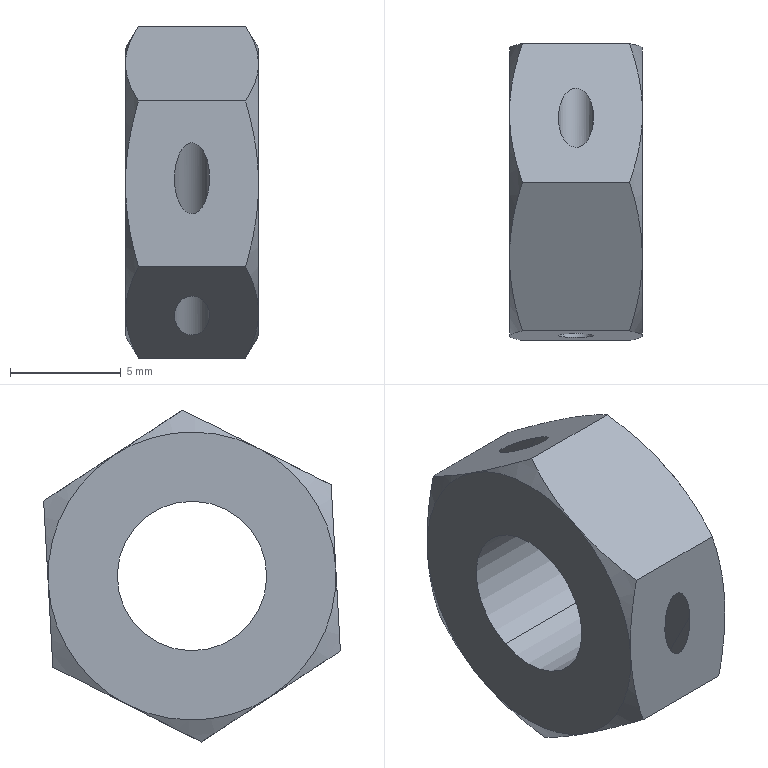Part | SolidWorks | features BaseBody 1 | 1 solid | 26 faces | box 6 x 13.398 x 14.988 mm | volume 630.737 mm3 | cone 12 | plane 8 | cylinder 6 | commonest cylinder face diameters 1.6 x4 6.75 x2
STEP:
#1=CARTESIAN_POINT('',(441.9,158.524,0.6198));
#2=VERTEX_POINT('',#1);
#3=CARTESIAN_POINT('',(440.3,158.524,0.6198));
#4=VERTEX_POINT('',#3);
#5=CARTESIAN_POINT('',(441.9,158.524,0.6198));
#6=CARTESIAN_POINT('',(441.9,158.346,-2.575));
#7=CARTESIAN_POINT('',(440.3,158.346,-2.575));
#8=CARTESIAN_POINT('',(440.3,158.524,0.6198));
#9=(BOUNDED_CURVE()B_SPLINE_CURVE(3,(#5,#6,#7,#8),.UNSPECIFIED.,.F.,.F.)B_SPLINE_CURVE_WITH_KNOTS((4,4),(4.712,7.854),.UNSPECIFIED.)CURVE()GEOMETRIC_REPRESENTATION_ITEM()RATIONAL_B_SPLINE_CURVE((1.,0.3333,0.3333,1.))REPRESENTATION_ITEM(''));
#10=EDGE_CURVE('',#2,#4,#9,.T.);
#11=ORIENTED_EDGE('',*,*,#10,.F.);
#12=CARTESIAN_POINT('',(441.9,161.658,-5.581));
#13=VERTEX_POINT('',#12);
#14=CARTESIAN_POINT('',(441.9,157.16,3.321));
#15=DIRECTION('',(0.,0.451,-0.8925));
#16=VECTOR('',#15,1000.);
#17=LINE('',#14,#16);
#18=EDGE_CURVE('',#2,#13,#17,.T.);
#19=ORIENTED_EDGE('',*,*,#18,.T.);
#20=CARTESIAN_POINT('',(440.3,161.658,-5.581));
#21=VERTEX_POINT('',#20);
#22=CARTESIAN_POINT('',(440.3,161.658,-5.581));
#23=CARTESIAN_POINT('',(440.3,158.98,-3.829));
#24=CARTESIAN_POINT('',(441.9,158.98,-3.829));
#25=CARTESIAN_POINT('',(441.9,161.658,-5.581));
#26=(BOUNDED_CURVE()B_SPLINE_CURVE(3,(#22,#23,#24,#25),.UNSPECIFIED.,.F.,.F.)B_SPLINE_CURVE_WITH_KNOTS((4,4),(1.571,4.712),.UNSPECIFIED.)CURVE()GEOMETRIC_REPRESENTATION_ITEM()RATIONAL_B_SPLINE_CURVE((1.,0.3333,0.3333,1.))REPRESENTATION_ITEM(''));
#27=EDGE_CURVE('',#21,#13,#26,.T.);
#28=ORIENTED_EDGE('',*,*,#27,.F.);
#29=CARTESIAN_POINT('',(440.3,157.16,3.321));
#30=DIRECTION('',(0.,0.451,-0.8925));
#31=VECTOR('',#30,1000.);
#32=LINE('',#29,#31);
#33=EDGE_CURVE('',#4,#21,#32,.T.);
#34=ORIENTED_EDGE('',*,*,#33,.F.);
#35=EDGE_LOOP('',(#11,#19,#28,#34));
#36=FACE_OUTER_BOUND('',#35,.T.);
#37=CARTESIAN_POINT('',(441.1,157.16,3.321));
#38=DIRECTION('',(0.,0.451,-0.8925));
#39=DIRECTION('',(-1.,0.,0.));
#40=AXIS2_PLACEMENT_3D('',#37,#38,#39);
#41=CYLINDRICAL_SURFACE('',#40,0.8);
#42=ADVANCED_FACE('',(#36),#41,.F.);
#43=CARTESIAN_POINT('',(441.9,168.342,5.581));
#44=VERTEX_POINT('',#43);
#45=CARTESIAN_POINT('',(440.3,168.342,5.581));
#46=VERTEX_POINT('',#45);
#47=CARTESIAN_POINT('',(441.9,168.342,5.581));
#48=CARTESIAN_POINT('',(441.9,165.664,7.333));
#49=CARTESIAN_POINT('',(440.3,165.664,7.333));
#50=CARTESIAN_POINT('',(440.3,168.342,5.581));
#51=(BOUNDED_CURVE()B_SPLINE_CURVE(3,(#47,#48,#49,#50),.UNSPECIFIED.,.F.,.T.)B_SPLINE_CURVE_WITH_KNOTS((4,4),(1.571,4.712),.UNSPECIFIED.)CURVE()GEOMETRIC_REPRESENTATION_ITEM()RATIONAL_B_SPLINE_CURVE((1.,0.3333,0.3333,1.))REPRESENTATION_ITEM(''));
#52=EDGE_CURVE('',#44,#46,#51,.T.);
#53=ORIENTED_EDGE('',*,*,#52,.F.);
#54=CARTESIAN_POINT('',(441.9,171.476,-0.6198));
#55=VERTEX_POINT('',#54);
#56=CARTESIAN_POINT('',(441.9,166.977,8.282));
#57=DIRECTION('',(0.,0.451,-0.8925));
#58=VECTOR('',#57,1000.);
#59=LINE('',#56,#58);
#60=EDGE_CURVE('',#44,#55,#59,.T.);
#61=ORIENTED_EDGE('',*,*,#60,.T.);
#62=CARTESIAN_POINT('',(440.3,171.476,-0.6198));
#63=VERTEX_POINT('',#62);
#64=CARTESIAN_POINT('',(440.3,171.476,-0.6198));
#65=CARTESIAN_POINT('',(440.3,171.297,-3.815));
#66=CARTESIAN_POINT('',(441.9,171.297,-3.815));
#67=CARTESIAN_POINT('',(441.9,171.476,-0.6198));
#68=(BOUNDED_CURVE()B_SPLINE_CURVE(3,(#64,#65,#66,#67),.UNSPECIFIED.,.F.,.T.)B_SPLINE_CURVE_WITH_KNOTS((4,4),(4.712,7.854),.UNSPECIFIED.)CURVE()GEOMETRIC_REPRESENTATION_ITEM()RATIONAL_B_SPLINE_CURVE((1.,0.3333,0.3333,1.))REPRESENTATION_ITEM(''));
#69=EDGE_CURVE('',#63,#55,#68,.T.);
#70=ORIENTED_EDGE('',*,*,#69,.F.);
#71=CARTESIAN_POINT('',(440.3,166.977,8.282));
#72=DIRECTION('',(0.,0.451,-0.8925));
#73=VECTOR('',#72,1000.);
#74=LINE('',#71,#73);
#75=EDGE_CURVE('',#46,#63,#74,.T.);
#76=ORIENTED_EDGE('',*,*,#75,.F.);
#77=EDGE_LOOP('',(#53,#61,#70,#76));
#78=FACE_OUTER_BOUND('',#77,.T.);
#79=CARTESIAN_POINT('',(441.1,166.977,8.282));
#80=DIRECTION('',(0.,0.451,-0.8925));
#81=DIRECTION('',(-1.,0.,0.));
#82=AXIS2_PLACEMENT_3D('',#79,#80,#81);
#83=CYLINDRICAL_SURFACE('',#82,0.8);
#84=ADVANCED_FACE('',(#78),#83,.F.);
#85=CARTESIAN_POINT('',(438.1,163.478,3.012));
#86=VERTEX_POINT('',#85);
#87=CARTESIAN_POINT('',(438.1,166.522,-3.012));
#88=VERTEX_POINT('',#87);
#89=CARTESIAN_POINT('',(438.1,165.,0.));
#90=DIRECTION('',(1.,0.,0.));
#91=DIRECTION('',(0.,0.451,-0.8925));
#92=AXIS2_PLACEMENT_3D('',#89,#90,#91);
#93=CIRCLE('',#92,3.375);
#94=EDGE_CURVE('',#86,#88,#93,.T.);
#95=ORIENTED_EDGE('',*,*,#94,.F.);
#96=CARTESIAN_POINT('',(444.1,163.478,3.012));
#97=VERTEX_POINT('',#96);
#98=CARTESIAN_POINT('',(438.1,163.478,3.012));
#99=DIRECTION('',(1.,0.,0.));
#100=VECTOR('',#99,1000.);
#101=LINE('',#98,#100);
#102=EDGE_CURVE('',#86,#97,#101,.T.);
#103=ORIENTED_EDGE('',*,*,#102,.T.);
#104=CARTESIAN_POINT('',(444.1,166.522,-3.012));
#105=VERTEX_POINT('',#104);
#106=CARTESIAN_POINT('',(444.1,165.,0.));
#107=DIRECTION('',(1.,0.,0.));
#108=DIRECTION('',(0.,0.451,-0.8925));
#109=AXIS2_PLACEMENT_3D('',#106,#107,#108);
#110=CIRCLE('',#109,3.375);
#111=EDGE_CURVE('',#97,#105,#110,.T.);
#112=ORIENTED_EDGE('',*,*,#111,.T.);
#113=CARTESIAN_POINT('',(438.1,166.522,-3.012));
#114=DIRECTION('',(1.,0.,0.));
#115=VECTOR('',#114,1000.);
#116=LINE('',#113,#115);
#117=EDGE_CURVE('',#88,#105,#116,.T.);
#118=ORIENTED_EDGE('',*,*,#117,.F.);
#119=EDGE_LOOP('',(#95,#103,#112,#118));
#120=FACE_OUTER_BOUND('',#119,.T.);
#121=CARTESIAN_POINT('',(438.1,165.,0.));
#122=DIRECTION('',(1.,0.,0.));
#123=DIRECTION('',(0.,0.451,-0.8925));
#124=AXIS2_PLACEMENT_3D('',#121,#122,#123);
#125=CYLINDRICAL_SURFACE('',#124,3.375);
#126=ADVANCED_FACE('',(#120),#125,.F.);
#127=ORIENTED_EDGE('',*,*,#69,.T.);
#128=CARTESIAN_POINT('',(441.9,171.476,-0.6198));
#129=CARTESIAN_POINT('',(441.9,171.654,2.575));
#130=CARTESIAN_POINT('',(440.3,171.654,2.575));
#131=CARTESIAN_POINT('',(440.3,171.476,-0.6198));
#132=(BOUNDED_CURVE()B_SPLINE_CURVE(3,(#128,#129,#130,#131),.UNSPECIFIED.,.F.,.F.)B_SPLINE_CURVE_WITH_KNOTS((4,4),(1.571,4.712),.UNSPECIFIED.)CURVE()GEOMETRIC_REPRESENTATION_ITEM()RATIONAL_B_SPLINE_CURVE((1.,0.3333,0.3333,1.))REPRESENTATION_ITEM(''));
#133=EDGE_CURVE('',#55,#63,#132,.T.);
#134=ORIENTED_EDGE('',*,*,#133,.T.);
#135=EDGE_LOOP('',(#127,#134));
#136=FACE_BOUND('',#135,.T.);
#137=CARTESIAN_POINT('',(438.681,171.699,3.385));
#138=VERTEX_POINT('',#137);
#139=CARTESIAN_POINT('',(438.1,171.49,-0.3619));
#140=VERTEX_POINT('',#139);
#141=CARTESIAN_POINT('',(438.681,171.699,3.385));
#142=CARTESIAN_POINT('',(438.503,171.665,2.772));
#143=CARTESIAN_POINT('',(438.357,171.63,2.155));
#144=CARTESIAN_POINT('',(438.155,171.561,0.9069));
#145=CARTESIAN_POINT('',(438.1,171.526,0.2765));
#146=CARTESIAN_POINT('',(438.1,171.49,-0.3619));
#147=B_SPLINE_CURVE_WITH_KNOTS('',3,(#141,#142,#143,#144,#145,#146),.UNSPECIFIED.,.F.,.F.,(4,2,4),(0.000000238,0.001899,0.003797),.UNSPECIFIED.);
#148=EDGE_CURVE('',#138,#140,#147,.T.);
#149=ORIENTED_EDGE('',*,*,#148,.F.);
#150=CARTESIAN_POINT('',(443.519,171.699,3.385));
#151=VERTEX_POINT('',#150);
#152=CARTESIAN_POINT('',(444.1,171.699,3.385));
#153=DIRECTION('',(-1.,0.,0.));
#154=VECTOR('',#153,1000.);
#155=LINE('',#152,#154);
#156=EDGE_CURVE('',#151,#138,#155,.T.);
#157=ORIENTED_EDGE('',*,*,#156,.F.);
#158=CARTESIAN_POINT('',(444.1,171.49,-0.3619));
#159=VERTEX_POINT('',#158);
#160=CARTESIAN_POINT('',(444.1,171.49,-0.3619));
#161=CARTESIAN_POINT('',(444.1,171.508,-0.04387));
#162=CARTESIAN_POINT('',(444.086,171.525,0.2755));
#163=CARTESIAN_POINT('',(444.033,171.561,0.9074));
#164=CARTESIAN_POINT('',(443.994,171.578,1.221));
#165=CARTESIAN_POINT('',(443.842,171.63,2.157));
#166=CARTESIAN_POINT('',(443.696,171.665,2.774));
#167=CARTESIAN_POINT('',(443.519,171.699,3.385));
#168=B_SPLINE_CURVE_WITH_KNOTS('',3,(#160,#161,#162,#163,#164,#165,#166,#167),.UNSPECIFIED.,.F.,.F.,(4,2,2,4),(0.003797,0.004743,0.005689,0.00758),.UNSPECIFIED.);
#169=EDGE_CURVE('',#159,#151,#168,.T.);
#170=ORIENTED_EDGE('',*,*,#169,.F.);
#171=CARTESIAN_POINT('',(443.519,171.281,-4.109));
#172=VERTEX_POINT('',#171);
#173=CARTESIAN_POINT('',(443.519,171.281,-4.109));
#174=CARTESIAN_POINT('',(443.697,171.315,-3.496));
#175=CARTESIAN_POINT('',(443.843,171.35,-2.878));
#176=CARTESIAN_POINT('',(444.045,171.419,-1.631));
#177=CARTESIAN_POINT('',(444.1,171.454,-1.));
#178=CARTESIAN_POINT('',(444.1,171.49,-0.3619));
#179=B_SPLINE_CURVE_WITH_KNOTS('',3,(#173,#174,#175,#176,#177,#178),.UNSPECIFIED.,.F.,.F.,(4,2,4),(0.000000238,0.001899,0.003797),.UNSPECIFIED.);
#180=EDGE_CURVE('',#172,#159,#179,.T.);
#181=ORIENTED_EDGE('',*,*,#180,.F.);
#182=CARTESIAN_POINT('',(438.681,171.281,-4.109));
#183=VERTEX_POINT('',#182);
#184=CARTESIAN_POINT('',(444.1,171.281,-4.109));
#185=DIRECTION('',(-1.,0.,0.));
#186=VECTOR('',#185,1000.);
#187=LINE('',#184,#186);
#188=EDGE_CURVE('',#172,#183,#187,.T.);
#189=ORIENTED_EDGE('',*,*,#188,.T.);
#190=CARTESIAN_POINT('',(438.1,171.49,-0.3619));
#191=CARTESIAN_POINT('',(438.1,171.472,-0.6799));
#192=CARTESIAN_POINT('',(438.114,171.454,-0.9993));
#193=CARTESIAN_POINT('',(438.167,171.419,-1.631));
#194=CARTESIAN_POINT('',(438.206,171.402,-1.945));
#195=CARTESIAN_POINT('',(438.358,171.349,-2.881));
#196=CARTESIAN_POINT('',(438.504,171.315,-3.497));
#197=CARTESIAN_POINT('',(438.681,171.281,-4.109));
#198=B_SPLINE_CURVE_WITH_KNOTS('',3,(#190,#191,#192,#193,#194,#195,#196,#197),.UNSPECIFIED.,.F.,.F.,(4,2,2,4),(0.003797,0.004743,0.005689,0.00758),.UNSPECIFIED.);
#199=EDGE_CURVE('',#140,#183,#198,.T.);
#200=ORIENTED_EDGE('',*,*,#199,.F.);
#201=EDGE_LOOP('',(#149,#157,#170,#181,#189,#200));
#202=FACE_OUTER_BOUND('',#201,.T.);
#203=CARTESIAN_POINT('',(444.1,171.281,-4.109));
#204=DIRECTION('',(0.,-0.9984,0.05567));
#205=DIRECTION('',(0.,-0.05567,-0.9984));
#206=AXIS2_PLACEMENT_3D('',#203,#204,#205);
#207=PLANE('',#206);
#208=ADVANCED_FACE('',(#136,#202),#207,.F.);
#209=CARTESIAN_POINT('',(440.3,168.342,5.581));
#210=CARTESIAN_POINT('',(440.3,171.02,3.829));
#211=CARTESIAN_POINT('',(441.9,171.02,3.829));
#212=CARTESIAN_POINT('',(441.9,168.342,5.581));
#213=(BOUNDED_CURVE()B_SPLINE_CURVE(3,(#209,#210,#211,#212),.UNSPECIFIED.,.F.,.F.)B_SPLINE_CURVE_WITH_KNOTS((4,4),(4.712,7.854),.UNSPECIFIED.)CURVE()GEOMETRIC_REPRESENTATION_ITEM()RATIONAL_B_SPLINE_CURVE((1.,0.3333,0.3333,1.))REPRESENTATION_ITEM(''));
#214=EDGE_CURVE('',#46,#44,#213,.T.);
#215=ORIENTED_EDGE('',*,*,#214,.T.);
#216=ORIENTED_EDGE('',*,*,#52,.T.);
#217=EDGE_LOOP('',(#215,#216));
#218=FACE_BOUND('',#217,.T.);
#219=CARTESIAN_POINT('',(438.681,165.418,7.494));
#220=VERTEX_POINT('',#219);
#221=CARTESIAN_POINT('',(438.1,168.558,5.44));
#222=VERTEX_POINT('',#221);
#223=CARTESIAN_POINT('',(438.681,165.418,7.494));
#224=CARTESIAN_POINT('',(438.503,165.932,7.158));
#225=CARTESIAN_POINT('',(438.357,166.449,6.819));
#226=CARTESIAN_POINT('',(438.155,167.495,6.135));
#227=CARTESIAN_POINT('',(438.1,168.023,5.79));
#228=CARTESIAN_POINT('',(438.1,168.558,5.44));
#229=B_SPLINE_CURVE_WITH_KNOTS('',3,(#223,#224,#225,#226,#227,#228),.UNSPECIFIED.,.F.,.F.,(4,2,4),(0.000000238,0.001899,0.003797),.UNSPECIFIED.);
#230=EDGE_CURVE('',#220,#222,#229,.T.);
#231=ORIENTED_EDGE('',*,*,#230,.F.);
#232=CARTESIAN_POINT('',(443.519,165.418,7.494));
#233=VERTEX_POINT('',#232);
#234=CARTESIAN_POINT('',(444.1,165.418,7.494));
#235=DIRECTION('',(-1.,0.,0.));
#236=VECTOR('',#235,1000.);
#237=LINE('',#234,#236);
#238=EDGE_CURVE('',#233,#220,#237,.T.);
#239=ORIENTED_EDGE('',*,*,#238,.F.);
#240=CARTESIAN_POINT('',(444.1,168.558,5.44));
#241=VERTEX_POINT('',#240);
#242=CARTESIAN_POINT('',(444.1,168.558,5.44));
#243=CARTESIAN_POINT('',(444.1,168.292,5.614));
#244=CARTESIAN_POINT('',(444.086,168.024,5.789));
#245=CARTESIAN_POINT('',(444.033,167.494,6.135));
#246=CARTESIAN_POINT('',(443.994,167.231,6.308));
#247=CARTESIAN_POINT('',(443.842,166.447,6.821));
#248=CARTESIAN_POINT('',(443.696,165.93,7.159));
#249=CARTESIAN_POINT('',(443.519,165.418,7.494));
#250=B_SPLINE_CURVE_WITH_KNOTS('',3,(#242,#243,#244,#245,#246,#247,#248,#249),.UNSPECIFIED.,.F.,.F.,(4,2,2,4),(0.003797,0.004743,0.005689,0.00758),.UNSPECIFIED.);
#251=EDGE_CURVE('',#241,#233,#250,.T.);
#252=ORIENTED_EDGE('',*,*,#251,.F.);
#253=CARTESIAN_POINT('',(443.519,171.699,3.385));
#254=CARTESIAN_POINT('',(443.697,171.185,3.721));
#255=CARTESIAN_POINT('',(443.843,170.668,4.06));
#256=CARTESIAN_POINT('',(444.045,169.622,4.744));
#257=CARTESIAN_POINT('',(444.1,169.093,5.089));
#258=CARTESIAN_POINT('',(444.1,168.558,5.44));
#259=B_SPLINE_CURVE_WITH_KNOTS('',3,(#253,#254,#255,#256,#257,#258),.UNSPECIFIED.,.F.,.F.,(4,2,4),(0.000000238,0.001899,0.003797),.UNSPECIFIED.);
#260=EDGE_CURVE('',#151,#241,#259,.T.);
#261=ORIENTED_EDGE('',*,*,#260,.F.);
#262=ORIENTED_EDGE('',*,*,#156,.T.);
#263=CARTESIAN_POINT('',(438.1,168.558,5.44));
#264=CARTESIAN_POINT('',(438.1,168.825,5.265));
#265=CARTESIAN_POINT('',(438.114,169.093,5.09));
#266=CARTESIAN_POINT('',(438.167,169.622,4.744));
#267=CARTESIAN_POINT('',(438.206,169.885,4.572));
#268=CARTESIAN_POINT('',(438.358,170.67,4.058));
#269=CARTESIAN_POINT('',(438.504,171.186,3.72));
#270=CARTESIAN_POINT('',(438.681,171.699,3.385));
#271=B_SPLINE_CURVE_WITH_KNOTS('',3,(#263,#264,#265,#266,#267,#268,#269,#270),.UNSPECIFIED.,.F.,.F.,(4,2,2,4),(0.003797,0.004743,0.005689,0.00758),.UNSPECIFIED.);
#272=EDGE_CURVE('',#222,#138,#271,.T.);
#273=ORIENTED_EDGE('',*,*,#272,.F.);
#274=EDGE_LOOP('',(#231,#239,#252,#261,#262,#273));
#275=FACE_OUTER_BOUND('',#274,.T.);
#276=CARTESIAN_POINT('',(444.1,171.699,3.385));
#277=DIRECTION('',(0.,-0.5474,-0.8368));
#278=DIRECTION('',(0.,0.8368,-0.5474));
#279=AXIS2_PLACEMENT_3D('',#276,#277,#278);
#280=PLANE('',#279);
#281=ADVANCED_FACE('',(#218,#275),#280,.F.);
#282=CARTESIAN_POINT('',(438.681,158.719,4.109));
#283=VERTEX_POINT('',#282);
#284=CARTESIAN_POINT('',(438.1,162.068,5.801));
#285=VERTEX_POINT('',#284);
#286=CARTESIAN_POINT('',(438.681,158.719,4.109));
#287=CARTESIAN_POINT('',(438.504,159.265,4.385));
#288=CARTESIAN_POINT('',(438.357,159.822,4.666));
#289=CARTESIAN_POINT('',(438.155,160.939,5.231));
#290=CARTESIAN_POINT('',(438.1,161.501,5.515));
#291=CARTESIAN_POINT('',(438.1,162.068,5.801));
#292=B_SPLINE_CURVE_WITH_KNOTS('',3,(#286,#287,#288,#289,#290,#291),.UNSPECIFIED.,.F.,.F.,(4,2,4),(0.007046,0.008945,0.01085),.UNSPECIFIED.);
#293=EDGE_CURVE('',#283,#285,#292,.T.);
#294=ORIENTED_EDGE('',*,*,#293,.F.);
#295=CARTESIAN_POINT('',(443.519,158.719,4.109));
#296=VERTEX_POINT('',#295);
#297=CARTESIAN_POINT('',(444.1,158.719,4.109));
#298=DIRECTION('',(-1.,0.,0.));
#299=VECTOR('',#298,1000.);
#300=LINE('',#297,#299);
#301=EDGE_CURVE('',#296,#283,#300,.T.);
#302=ORIENTED_EDGE('',*,*,#301,.F.);
#303=CARTESIAN_POINT('',(444.1,162.068,5.801));
#304=VERTEX_POINT('',#303);
#305=CARTESIAN_POINT('',(444.1,162.068,5.801));
#306=CARTESIAN_POINT('',(444.1,161.501,5.515));
#307=CARTESIAN_POINT('',(444.045,160.939,5.231));
#308=CARTESIAN_POINT('',(443.843,159.822,4.666));
#309=CARTESIAN_POINT('',(443.696,159.265,4.385));
#310=CARTESIAN_POINT('',(443.519,158.719,4.109));
#311=B_SPLINE_CURVE_WITH_KNOTS('',3,(#305,#306,#307,#308,#309,#310),.UNSPECIFIED.,.F.,.F.,(4,2,4),(0.02413,0.02603,0.02793),.UNSPECIFIED.);
#312=EDGE_CURVE('',#304,#296,#311,.T.);
#313=ORIENTED_EDGE('',*,*,#312,.F.);
#314=CARTESIAN_POINT('',(443.519,165.418,7.494));
#315=CARTESIAN_POINT('',(443.695,164.876,7.22));
#316=CARTESIAN_POINT('',(443.84,164.327,6.943));
#317=CARTESIAN_POINT('',(443.993,163.489,6.519));
#318=CARTESIAN_POINT('',(444.033,163.208,6.377));
#319=CARTESIAN_POINT('',(444.086,162.638,6.089));
#320=CARTESIAN_POINT('',(444.1,162.352,5.945));
#321=CARTESIAN_POINT('',(444.1,162.068,5.801));
#322=B_SPLINE_CURVE_WITH_KNOTS('',3,(#314,#315,#316,#317,#318,#319,#320,#321),.UNSPECIFIED.,.F.,.F.,(4,2,2,4),(0.02033,0.02223,0.02318,0.02413),.UNSPECIFIED.);
#323=EDGE_CURVE('',#233,#304,#322,.T.);
#324=ORIENTED_EDGE('',*,*,#323,.F.);
#325=ORIENTED_EDGE('',*,*,#238,.T.);
#326=CARTESIAN_POINT('',(438.1,162.068,5.801));
#327=CARTESIAN_POINT('',(438.1,162.352,5.945));
#328=CARTESIAN_POINT('',(438.114,162.638,6.089));
#329=CARTESIAN_POINT('',(438.167,163.208,6.377));
#330=CARTESIAN_POINT('',(438.207,163.489,6.519));
#331=CARTESIAN_POINT('',(438.36,164.327,6.943));
#332=CARTESIAN_POINT('',(438.505,164.876,7.22));
#333=CARTESIAN_POINT('',(438.681,165.418,7.494));
#334=B_SPLINE_CURVE_WITH_KNOTS('',3,(#326,#327,#328,#329,#330,#331,#332,#333),.UNSPECIFIED.,.F.,.F.,(4,2,2,4),(0.01085,0.0118,0.01275,0.01465),.UNSPECIFIED.);
#335=EDGE_CURVE('',#285,#220,#334,.T.);
#336=ORIENTED_EDGE('',*,*,#335,.F.);
#337=EDGE_LOOP('',(#294,#302,#313,#324,#325,#336));
#338=FACE_OUTER_BOUND('',#337,.T.);
#339=CARTESIAN_POINT('',(444.1,165.418,7.494));
#340=DIRECTION('',(0.,0.451,-0.8925));
#341=DIRECTION('',(0.,0.8925,0.451));
#342=AXIS2_PLACEMENT_3D('',#339,#340,#341);
#343=PLANE('',#342);
#344=ADVANCED_FACE('',(#338),#343,.F.);
#345=CARTESIAN_POINT('',(440.3,158.524,0.6198));
#346=CARTESIAN_POINT('',(440.3,158.703,3.815));
#347=CARTESIAN_POINT('',(441.9,158.703,3.815));
#348=CARTESIAN_POINT('',(441.9,158.524,0.6198));
#349=(BOUNDED_CURVE()B_SPLINE_CURVE(3,(#345,#346,#347,#348),.UNSPECIFIED.,.F.,.F.)B_SPLINE_CURVE_WITH_KNOTS((4,4),(1.571,4.712),.UNSPECIFIED.)CURVE()GEOMETRIC_REPRESENTATION_ITEM()RATIONAL_B_SPLINE_CURVE((1.,0.3333,0.3333,1.))REPRESENTATION_ITEM(''));
#350=EDGE_CURVE('',#4,#2,#349,.T.);
#351=ORIENTED_EDGE('',*,*,#350,.T.);
#352=ORIENTED_EDGE('',*,*,#10,.T.);
#353=EDGE_LOOP('',(#351,#352));
#354=FACE_BOUND('',#353,.T.);
#355=CARTESIAN_POINT('',(438.681,158.301,-3.385));
#356=VERTEX_POINT('',#355);
#357=CARTESIAN_POINT('',(438.1,158.51,0.3619));
#358=VERTEX_POINT('',#357);
#359=CARTESIAN_POINT('',(438.681,158.301,-3.385));
#360=CARTESIAN_POINT('',(438.503,158.335,-2.772));
#361=CARTESIAN_POINT('',(438.357,158.37,-2.155));
#362=CARTESIAN_POINT('',(438.155,158.439,-0.9069));
#363=CARTESIAN_POINT('',(438.1,158.474,-0.2765));
#364=CARTESIAN_POINT('',(438.1,158.51,0.3619));
#365=B_SPLINE_CURVE_WITH_KNOTS('',3,(#359,#360,#361,#362,#363,#364),.UNSPECIFIED.,.F.,.F.,(4,2,4),(0.000000238,0.001899,0.003797),.UNSPECIFIED.);
#366=EDGE_CURVE('',#356,#358,#365,.T.);
#367=ORIENTED_EDGE('',*,*,#366,.F.);
#368=CARTESIAN_POINT('',(443.519,158.301,-3.385));
#369=VERTEX_POINT('',#368);
#370=CARTESIAN_POINT('',(444.1,158.301,-3.385));
#371=DIRECTION('',(-1.,0.,0.));
#372=VECTOR('',#371,1000.);
#373=LINE('',#370,#372);
#374=EDGE_CURVE('',#369,#356,#373,.T.);
#375=ORIENTED_EDGE('',*,*,#374,.F.);
#376=CARTESIAN_POINT('',(444.1,158.51,0.3619));
#377=VERTEX_POINT('',#376);
#378=CARTESIAN_POINT('',(444.1,158.51,0.3619));
#379=CARTESIAN_POINT('',(444.1,158.492,0.04387));
#380=CARTESIAN_POINT('',(444.086,158.475,-0.2755));
#381=CARTESIAN_POINT('',(444.033,158.439,-0.9074));
#382=CARTESIAN_POINT('',(443.994,158.422,-1.221));
#383=CARTESIAN_POINT('',(443.842,158.37,-2.157));
#384=CARTESIAN_POINT('',(443.696,158.335,-2.774));
#385=CARTESIAN_POINT('',(443.519,158.301,-3.385));
#386=B_SPLINE_CURVE_WITH_KNOTS('',3,(#378,#379,#380,#381,#382,#383,#384,#385),.UNSPECIFIED.,.F.,.F.,(4,2,2,4),(0.003797,0.004743,0.005689,0.00758),.UNSPECIFIED.);
#387=EDGE_CURVE('',#377,#369,#386,.T.);
#388=ORIENTED_EDGE('',*,*,#387,.F.);
#389=CARTESIAN_POINT('',(443.519,158.719,4.109));
#390=CARTESIAN_POINT('',(443.697,158.685,3.496));
#391=CARTESIAN_POINT('',(443.843,158.65,2.878));
#392=CARTESIAN_POINT('',(444.045,158.581,1.631));
#393=CARTESIAN_POINT('',(444.1,158.546,1.));
#394=CARTESIAN_POINT('',(444.1,158.51,0.3619));
#395=B_SPLINE_CURVE_WITH_KNOTS('',3,(#389,#390,#391,#392,#393,#394),.UNSPECIFIED.,.F.,.F.,(4,2,4),(0.000000238,0.001899,0.003797),.UNSPECIFIED.);
#396=EDGE_CURVE('',#296,#377,#395,.T.);
#397=ORIENTED_EDGE('',*,*,#396,.F.);
#398=ORIENTED_EDGE('',*,*,#301,.T.);
#399=CARTESIAN_POINT('',(438.1,158.51,0.3619));
#400=CARTESIAN_POINT('',(438.1,158.528,0.6799));
#401=CARTESIAN_POINT('',(438.114,158.546,0.9993));
#402=CARTESIAN_POINT('',(438.167,158.581,1.631));
#403=CARTESIAN_POINT('',(438.206,158.598,1.945));
#404=CARTESIAN_POINT('',(438.358,158.651,2.881));
#405=CARTESIAN_POINT('',(438.504,158.685,3.497));
#406=CARTESIAN_POINT('',(438.681,158.719,4.109));
#407=B_SPLINE_CURVE_WITH_KNOTS('',3,(#399,#400,#401,#402,#403,#404,#405,#406),.UNSPECIFIED.,.F.,.F.,(4,2,2,4),(0.003797,0.004743,0.005689,0.00758),.UNSPECIFIED.);
#408=EDGE_CURVE('',#358,#283,#407,.T.);
#409=ORIENTED_EDGE('',*,*,#408,.F.);
#410=EDGE_LOOP('',(#367,#375,#388,#397,#398,#409));
#411=FACE_OUTER_BOUND('',#410,.T.);
#412=CARTESIAN_POINT('',(444.1,158.719,4.109));
#413=DIRECTION('',(0.,0.9984,-0.05567));
#414=DIRECTION('',(0.,0.05567,0.9984));
#415=AXIS2_PLACEMENT_3D('',#412,#413,#414);
#416=PLANE('',#415);
#417=ADVANCED_FACE('',(#354,#411),#416,.F.);
#418=ORIENTED_EDGE('',*,*,#27,.T.);
#419=CARTESIAN_POINT('',(441.9,161.658,-5.581));
#420=CARTESIAN_POINT('',(441.9,164.336,-7.333));
#421=CARTESIAN_POINT('',(440.3,164.336,-7.333));
#422=CARTESIAN_POINT('',(440.3,161.658,-5.581));
#423=(BOUNDED_CURVE()B_SPLINE_CURVE(3,(#419,#420,#421,#422),.UNSPECIFIED.,.F.,.T.)B_SPLINE_CURVE_WITH_KNOTS((4,4),(4.712,7.854),.UNSPECIFIED.)CURVE()GEOMETRIC_REPRESENTATION_ITEM()RATIONAL_B_SPLINE_CURVE((1.,0.3333,0.3333,1.))REPRESENTATION_ITEM(''));
#424=EDGE_CURVE('',#13,#21,#423,.T.);
#425=ORIENTED_EDGE('',*,*,#424,.T.);
#426=EDGE_LOOP('',(#418,#425));
#427=FACE_BOUND('',#426,.T.);
#428=CARTESIAN_POINT('',(438.681,164.582,-7.494));
#429=VERTEX_POINT('',#428);
#430=CARTESIAN_POINT('',(438.1,161.442,-5.44));
#431=VERTEX_POINT('',#430);
#432=CARTESIAN_POINT('',(438.681,164.582,-7.494));
#433=CARTESIAN_POINT('',(438.503,164.068,-7.158));
#434=CARTESIAN_POINT('',(438.357,163.551,-6.819));
#435=CARTESIAN_POINT('',(438.155,162.505,-6.135));
#436=CARTESIAN_POINT('',(438.1,161.977,-5.79));
#437=CARTESIAN_POINT('',(438.1,161.442,-5.44));
#438=B_SPLINE_CURVE_WITH_KNOTS('',3,(#432,#433,#434,#435,#436,#437),.UNSPECIFIED.,.F.,.F.,(4,2,4),(0.000000238,0.001899,0.003797),.UNSPECIFIED.);
#439=EDGE_CURVE('',#429,#431,#438,.T.);
#440=ORIENTED_EDGE('',*,*,#439,.F.);
#441=CARTESIAN_POINT('',(443.519,164.582,-7.494));
#442=VERTEX_POINT('',#441);
#443=CARTESIAN_POINT('',(444.1,164.582,-7.494));
#444=DIRECTION('',(-1.,0.,0.));
#445=VECTOR('',#444,1000.);
#446=LINE('',#443,#445);
#447=EDGE_CURVE('',#442,#429,#446,.T.);
#448=ORIENTED_EDGE('',*,*,#447,.F.);
#449=CARTESIAN_POINT('',(444.1,161.442,-5.44));
#450=VERTEX_POINT('',#449);
#451=CARTESIAN_POINT('',(444.1,161.442,-5.44));
#452=CARTESIAN_POINT('',(444.1,161.708,-5.614));
#453=CARTESIAN_POINT('',(444.086,161.976,-5.789));
#454=CARTESIAN_POINT('',(444.033,162.506,-6.135));
#455=CARTESIAN_POINT('',(443.994,162.769,-6.308));
#456=CARTESIAN_POINT('',(443.842,163.553,-6.821));
#457=CARTESIAN_POINT('',(443.696,164.07,-7.159));
#458=CARTESIAN_POINT('',(443.519,164.582,-7.494));
#459=B_SPLINE_CURVE_WITH_KNOTS('',3,(#451,#452,#453,#454,#455,#456,#457,#458),.UNSPECIFIED.,.F.,.F.,(4,2,2,4),(0.003797,0.004743,0.005689,0.00758),.UNSPECIFIED.);
#460=EDGE_CURVE('',#450,#442,#459,.T.);
#461=ORIENTED_EDGE('',*,*,#460,.F.);
#462=CARTESIAN_POINT('',(443.519,158.301,-3.385));
#463=CARTESIAN_POINT('',(443.697,158.815,-3.721));
#464=CARTESIAN_POINT('',(443.843,159.332,-4.06));
#465=CARTESIAN_POINT('',(444.045,160.378,-4.744));
#466=CARTESIAN_POINT('',(444.1,160.907,-5.089));
#467=CARTESIAN_POINT('',(444.1,161.442,-5.44));
#468=B_SPLINE_CURVE_WITH_KNOTS('',3,(#462,#463,#464,#465,#466,#467),.UNSPECIFIED.,.F.,.F.,(4,2,4),(0.000000238,0.001899,0.003797),.UNSPECIFIED.);
#469=EDGE_CURVE('',#369,#450,#468,.T.);
#470=ORIENTED_EDGE('',*,*,#469,.F.);
#471=ORIENTED_EDGE('',*,*,#374,.T.);
#472=CARTESIAN_POINT('',(438.1,161.442,-5.44));
#473=CARTESIAN_POINT('',(438.1,161.175,-5.265));
#474=CARTESIAN_POINT('',(438.114,160.907,-5.09));
#475=CARTESIAN_POINT('',(438.167,160.378,-4.744));
#476=CARTESIAN_POINT('',(438.206,160.115,-4.572));
#477=CARTESIAN_POINT('',(438.358,159.33,-4.058));
#478=CARTESIAN_POINT('',(438.504,158.814,-3.72));
#479=CARTESIAN_POINT('',(438.681,158.301,-3.385));
#480=B_SPLINE_CURVE_WITH_KNOTS('',3,(#472,#473,#474,#475,#476,#477,#478,#479),.UNSPECIFIED.,.F.,.F.,(4,2,2,4),(0.003797,0.004743,0.005689,0.00758),.UNSPECIFIED.);
#481=EDGE_CURVE('',#431,#356,#480,.T.);
#482=ORIENTED_EDGE('',*,*,#481,.F.);
#483=EDGE_LOOP('',(#440,#448,#461,#470,#471,#482));
#484=FACE_OUTER_BOUND('',#483,.T.);
#485=CARTESIAN_POINT('',(444.1,158.301,-3.385));
#486=DIRECTION('',(0.,0.5474,0.8368));
#487=DIRECTION('',(0.,-0.8368,0.5474));
#488=AXIS2_PLACEMENT_3D('',#485,#486,#487);
#489=PLANE('',#488);
#490=ADVANCED_FACE('',(#427,#484),#489,.F.);
#491=CARTESIAN_POINT('',(438.1,167.932,-5.801));
#492=VERTEX_POINT('',#491);
#493=CARTESIAN_POINT('',(438.681,171.281,-4.109));
#494=CARTESIAN_POINT('',(438.505,170.739,-4.383));
#495=CARTESIAN_POINT('',(438.36,170.191,-4.66));
#496=CARTESIAN_POINT('',(438.207,169.353,-5.083));
#497=CARTESIAN_POINT('',(438.167,169.071,-5.226));
#498=CARTESIAN_POINT('',(438.114,168.501,-5.514));
#499=CARTESIAN_POINT('',(438.1,168.215,-5.658));
#500=CARTESIAN_POINT('',(438.1,167.932,-5.801));
#501=B_SPLINE_CURVE_WITH_KNOTS('',3,(#493,#494,#495,#496,#497,#498,#499,#500),.UNSPECIFIED.,.F.,.F.,(4,2,2,4),(0.02033,0.02223,0.02318,0.02413),.UNSPECIFIED.);
#502=EDGE_CURVE('',#183,#492,#501,.T.);
#503=ORIENTED_EDGE('',*,*,#502,.F.);
#504=ORIENTED_EDGE('',*,*,#188,.F.);
#505=CARTESIAN_POINT('',(444.1,167.932,-5.801));
#506=VERTEX_POINT('',#505);
#507=CARTESIAN_POINT('',(444.1,167.932,-5.801));
#508=CARTESIAN_POINT('',(444.1,168.215,-5.658));
#509=CARTESIAN_POINT('',(444.086,168.501,-5.514));
#510=CARTESIAN_POINT('',(444.033,169.071,-5.226));
#511=CARTESIAN_POINT('',(443.993,169.353,-5.083));
#512=CARTESIAN_POINT('',(443.84,170.191,-4.66));
#513=CARTESIAN_POINT('',(443.695,170.739,-4.383));
#514=CARTESIAN_POINT('',(443.519,171.281,-4.109));
#515=B_SPLINE_CURVE_WITH_KNOTS('',3,(#507,#508,#509,#510,#511,#512,#513,#514),.UNSPECIFIED.,.F.,.F.,(4,2,2,4),(0.01085,0.0118,0.01275,0.01465),.UNSPECIFIED.);
#516=EDGE_CURVE('',#506,#172,#515,.T.);
#517=ORIENTED_EDGE('',*,*,#516,.F.);
#518=CARTESIAN_POINT('',(443.519,164.582,-7.494));
#519=CARTESIAN_POINT('',(443.696,165.128,-7.218));
#520=CARTESIAN_POINT('',(443.843,165.685,-6.937));
#521=CARTESIAN_POINT('',(444.045,166.802,-6.372));
#522=CARTESIAN_POINT('',(444.1,167.365,-6.088));
#523=CARTESIAN_POINT('',(444.1,167.932,-5.801));
#524=B_SPLINE_CURVE_WITH_KNOTS('',3,(#518,#519,#520,#521,#522,#523),.UNSPECIFIED.,.F.,.F.,(4,2,4),(0.007046,0.008945,0.01085),.UNSPECIFIED.);
#525=EDGE_CURVE('',#442,#506,#524,.T.);
#526=ORIENTED_EDGE('',*,*,#525,.F.);
#527=ORIENTED_EDGE('',*,*,#447,.T.);
#528=CARTESIAN_POINT('',(438.1,167.932,-5.801));
#529=CARTESIAN_POINT('',(438.1,167.365,-6.088));
#530=CARTESIAN_POINT('',(438.155,166.802,-6.372));
#531=CARTESIAN_POINT('',(438.357,165.685,-6.937));
#532=CARTESIAN_POINT('',(438.504,165.128,-7.218));
#533=CARTESIAN_POINT('',(438.681,164.582,-7.494));
#534=B_SPLINE_CURVE_WITH_KNOTS('',3,(#528,#529,#530,#531,#532,#533),.UNSPECIFIED.,.F.,.F.,(4,2,4),(0.02413,0.02603,0.02793),.UNSPECIFIED.);
#535=EDGE_CURVE('',#492,#429,#534,.T.);
#536=ORIENTED_EDGE('',*,*,#535,.F.);
#537=EDGE_LOOP('',(#503,#504,#517,#526,#527,#536));
#538=FACE_OUTER_BOUND('',#537,.T.);
#539=CARTESIAN_POINT('',(444.1,164.582,-7.494));
#540=DIRECTION('',(0.,-0.451,0.8925));
#541=DIRECTION('',(1.,0.,0.));
#542=AXIS2_PLACEMENT_3D('',#539,#540,#541);
#543=PLANE('',#542);
#544=ADVANCED_FACE('',(#538),#543,.F.);
#545=ORIENTED_EDGE('',*,*,#312,.T.);
#546=ORIENTED_EDGE('',*,*,#396,.T.);
#547=CARTESIAN_POINT('',(444.1,165.,0.));
#548=DIRECTION('',(-1.,0.,0.));
#549=DIRECTION('',(0.,-0.451,0.8925));
#550=AXIS2_PLACEMENT_3D('',#547,#548,#549);
#551=CIRCLE('',#550,6.5);
#552=EDGE_CURVE('',#377,#304,#551,.T.);
#553=ORIENTED_EDGE('',*,*,#552,.T.);
#554=EDGE_LOOP('',(#545,#546,#553));
#555=FACE_OUTER_BOUND('',#554,.T.);
#556=CARTESIAN_POINT('',(444.1,165.,0.));
#557=DIRECTION('',(-1.,0.,0.));
#558=DIRECTION('',(0.,0.451,-0.8925));
#559=AXIS2_PLACEMENT_3D('',#556,#557,#558);
#560=CONICAL_SURFACE('',#559,6.5,1.047);
#561=ADVANCED_FACE('',(#555),#560,.T.);
#562=ORIENTED_EDGE('',*,*,#387,.T.);
#563=ORIENTED_EDGE('',*,*,#469,.T.);
#564=CARTESIAN_POINT('',(444.1,165.,0.));
#565=DIRECTION('',(-1.,0.,0.));
#566=DIRECTION('',(0.,-0.451,0.8925));
#567=AXIS2_PLACEMENT_3D('',#564,#565,#566);
#568=CIRCLE('',#567,6.5);
#569=EDGE_CURVE('',#450,#377,#568,.T.);
#570=ORIENTED_EDGE('',*,*,#569,.T.);
#571=EDGE_LOOP('',(#562,#563,#570));
#572=FACE_OUTER_BOUND('',#571,.T.);
#573=CARTESIAN_POINT('',(444.1,165.,0.));
#574=DIRECTION('',(-1.,0.,0.));
#575=DIRECTION('',(0.,0.451,-0.8925));
#576=AXIS2_PLACEMENT_3D('',#573,#574,#575);
#577=CONICAL_SURFACE('',#576,6.5,1.047);
#578=ADVANCED_FACE('',(#572),#577,.T.);
#579=ORIENTED_EDGE('',*,*,#460,.T.);
#580=ORIENTED_EDGE('',*,*,#525,.T.);
#581=CARTESIAN_POINT('',(444.1,165.,0.));
#582=DIRECTION('',(-1.,0.,0.));
#583=DIRECTION('',(0.,-0.451,0.8925));
#584=AXIS2_PLACEMENT_3D('',#581,#582,#583);
#585=CIRCLE('',#584,6.5);
#586=EDGE_CURVE('',#506,#450,#585,.T.);
#587=ORIENTED_EDGE('',*,*,#586,.T.);
#588=EDGE_LOOP('',(#579,#580,#587));
#589=FACE_OUTER_BOUND('',#588,.T.);
#590=CARTESIAN_POINT('',(444.1,165.,0.));
#591=DIRECTION('',(-1.,0.,0.));
#592=DIRECTION('',(0.,0.451,-0.8925));
#593=AXIS2_PLACEMENT_3D('',#590,#591,#592);
#594=CONICAL_SURFACE('',#593,6.5,1.047);
#595=ADVANCED_FACE('',(#589),#594,.T.);
#596=ORIENTED_EDGE('',*,*,#180,.T.);
#597=CARTESIAN_POINT('',(444.1,165.,0.));
#598=DIRECTION('',(1.,0.,0.));
#599=DIRECTION('',(0.,0.451,-0.8925));
#600=AXIS2_PLACEMENT_3D('',#597,#598,#599);
#601=CIRCLE('',#600,6.5);
#602=EDGE_CURVE('',#506,#159,#601,.T.);
#603=ORIENTED_EDGE('',*,*,#602,.F.);
#604=ORIENTED_EDGE('',*,*,#516,.T.);
#605=EDGE_LOOP('',(#596,#603,#604));
#606=FACE_OUTER_BOUND('',#605,.T.);
#607=CARTESIAN_POINT('',(444.1,165.,0.));
#608=DIRECTION('',(-1.,0.,0.));
#609=DIRECTION('',(0.,0.451,-0.8925));
#610=AXIS2_PLACEMENT_3D('',#607,#608,#609);
#611=CONICAL_SURFACE('',#610,6.5,1.047);
#612=ADVANCED_FACE('',(#606),#611,.T.);
#613=ORIENTED_EDGE('',*,*,#169,.T.);
#614=ORIENTED_EDGE('',*,*,#260,.T.);
#615=CARTESIAN_POINT('',(444.1,165.,0.));
#616=DIRECTION('',(-1.,0.,0.));
#617=DIRECTION('',(0.,-0.451,0.8925));
#618=AXIS2_PLACEMENT_3D('',#615,#616,#617);
#619=CIRCLE('',#618,6.5);
#620=EDGE_CURVE('',#241,#159,#619,.T.);
#621=ORIENTED_EDGE('',*,*,#620,.T.);
#622=EDGE_LOOP('',(#613,#614,#621));
#623=FACE_OUTER_BOUND('',#622,.T.);
#624=CARTESIAN_POINT('',(444.1,165.,0.));
#625=DIRECTION('',(-1.,0.,0.));
#626=DIRECTION('',(0.,0.451,-0.8925));
#627=AXIS2_PLACEMENT_3D('',#624,#625,#626);
#628=CONICAL_SURFACE('',#627,6.5,1.047);
#629=ADVANCED_FACE('',(#623),#628,.T.);
#630=ORIENTED_EDGE('',*,*,#251,.T.);
#631=ORIENTED_EDGE('',*,*,#323,.T.);
#632=CARTESIAN_POINT('',(444.1,165.,0.));
#633=DIRECTION('',(-1.,0.,0.));
#634=DIRECTION('',(0.,-0.451,0.8925));
#635=AXIS2_PLACEMENT_3D('',#632,#633,#634);
#636=CIRCLE('',#635,6.5);
#637=EDGE_CURVE('',#304,#241,#636,.T.);
#638=ORIENTED_EDGE('',*,*,#637,.T.);
#639=EDGE_LOOP('',(#630,#631,#638));
#640=FACE_OUTER_BOUND('',#639,.T.);
#641=CARTESIAN_POINT('',(444.1,165.,0.));
#642=DIRECTION('',(-1.,0.,0.));
#643=DIRECTION('',(0.,0.451,-0.8925));
#644=AXIS2_PLACEMENT_3D('',#641,#642,#643);
#645=CONICAL_SURFACE('',#644,6.5,1.047);
#646=ADVANCED_FACE('',(#640),#645,.T.);
#647=CARTESIAN_POINT('',(444.1,165.,0.));
#648=DIRECTION('',(1.,0.,0.));
#649=DIRECTION('',(0.,0.451,-0.8925));
#650=AXIS2_PLACEMENT_3D('',#647,#648,#649);
#651=CIRCLE('',#650,3.375);
#652=EDGE_CURVE('',#105,#97,#651,.T.);
#653=ORIENTED_EDGE('',*,*,#652,.F.);
#654=ORIENTED_EDGE('',*,*,#111,.F.);
#655=EDGE_LOOP('',(#653,#654));
#656=FACE_BOUND('',#655,.T.);
#657=ORIENTED_EDGE('',*,*,#637,.F.);
#658=ORIENTED_EDGE('',*,*,#552,.F.);
#659=ORIENTED_EDGE('',*,*,#569,.F.);
#660=ORIENTED_EDGE('',*,*,#586,.F.);
#661=ORIENTED_EDGE('',*,*,#602,.T.);
#662=ORIENTED_EDGE('',*,*,#620,.F.);
#663=EDGE_LOOP('',(#657,#658,#659,#660,#661,#662));
#664=FACE_OUTER_BOUND('',#663,.T.);
#665=CARTESIAN_POINT('',(444.1,170.863,-11.603));
#666=DIRECTION('',(-1.,0.,0.));
#667=DIRECTION('',(0.,-0.451,0.8925));
#668=AXIS2_PLACEMENT_3D('',#665,#666,#667);
#669=PLANE('',#668);
#670=ADVANCED_FACE('',(#656,#664),#669,.F.);
#671=ORIENTED_EDGE('',*,*,#293,.T.);
#672=CARTESIAN_POINT('',(438.1,165.,0.));
#673=DIRECTION('',(-1.,0.,0.));
#674=DIRECTION('',(0.,-0.451,0.8925));
#675=AXIS2_PLACEMENT_3D('',#672,#673,#674);
#676=CIRCLE('',#675,6.5);
#677=EDGE_CURVE('',#358,#285,#676,.T.);
#678=ORIENTED_EDGE('',*,*,#677,.F.);
#679=ORIENTED_EDGE('',*,*,#408,.T.);
#680=EDGE_LOOP('',(#671,#678,#679));
#681=FACE_OUTER_BOUND('',#680,.T.);
#682=CARTESIAN_POINT('',(438.1,165.,0.));
#683=DIRECTION('',(1.,0.,0.));
#684=DIRECTION('',(0.,-0.451,0.8925));
#685=AXIS2_PLACEMENT_3D('',#682,#683,#684);
#686=CONICAL_SURFACE('',#685,6.5,1.047);
#687=ADVANCED_FACE('',(#681),#686,.T.);
#688=ORIENTED_EDGE('',*,*,#366,.T.);
#689=CARTESIAN_POINT('',(438.1,165.,0.));
#690=DIRECTION('',(-1.,0.,0.));
#691=DIRECTION('',(0.,-0.451,0.8925));
#692=AXIS2_PLACEMENT_3D('',#689,#690,#691);
#693=CIRCLE('',#692,6.5);
#694=EDGE_CURVE('',#431,#358,#693,.T.);
#695=ORIENTED_EDGE('',*,*,#694,.F.);
#696=ORIENTED_EDGE('',*,*,#481,.T.);
#697=EDGE_LOOP('',(#688,#695,#696));
#698=FACE_OUTER_BOUND('',#697,.T.);
#699=CARTESIAN_POINT('',(438.1,165.,0.));
#700=DIRECTION('',(1.,0.,0.));
#701=DIRECTION('',(0.,-0.451,0.8925));
#702=AXIS2_PLACEMENT_3D('',#699,#700,#701);
#703=CONICAL_SURFACE('',#702,6.5,1.047);
#704=ADVANCED_FACE('',(#698),#703,.T.);
#705=ORIENTED_EDGE('',*,*,#439,.T.);
#706=CARTESIAN_POINT('',(438.1,165.,0.));
#707=DIRECTION('',(-1.,0.,0.));
#708=DIRECTION('',(0.,-0.451,0.8925));
#709=AXIS2_PLACEMENT_3D('',#706,#707,#708);
#710=CIRCLE('',#709,6.5);
#711=EDGE_CURVE('',#492,#431,#710,.T.);
#712=ORIENTED_EDGE('',*,*,#711,.F.);
#713=ORIENTED_EDGE('',*,*,#535,.T.);
#714=EDGE_LOOP('',(#705,#712,#713));
#715=FACE_OUTER_BOUND('',#714,.T.);
#716=CARTESIAN_POINT('',(438.1,165.,0.));
#717=DIRECTION('',(1.,0.,0.));
#718=DIRECTION('',(0.,-0.451,0.8925));
#719=AXIS2_PLACEMENT_3D('',#716,#717,#718);
#720=CONICAL_SURFACE('',#719,6.5,1.047);
#721=ADVANCED_FACE('',(#715),#720,.T.);
#722=ORIENTED_EDGE('',*,*,#199,.T.);
#723=ORIENTED_EDGE('',*,*,#502,.T.);
#724=CARTESIAN_POINT('',(438.1,165.,0.));
#725=DIRECTION('',(-1.,0.,0.));
#726=DIRECTION('',(0.,-0.451,0.8925));
#727=AXIS2_PLACEMENT_3D('',#724,#725,#726);
#728=CIRCLE('',#727,6.5);
#729=EDGE_CURVE('',#140,#492,#728,.T.);
#730=ORIENTED_EDGE('',*,*,#729,.F.);
#731=EDGE_LOOP('',(#722,#723,#730));
#732=FACE_OUTER_BOUND('',#731,.T.);
#733=CARTESIAN_POINT('',(438.1,165.,0.));
#734=DIRECTION('',(1.,0.,0.));
#735=DIRECTION('',(0.,-0.451,0.8925));
#736=AXIS2_PLACEMENT_3D('',#733,#734,#735);
#737=CONICAL_SURFACE('',#736,6.5,1.047);
#738=ADVANCED_FACE('',(#732),#737,.T.);
#739=ORIENTED_EDGE('',*,*,#272,.T.);
#740=ORIENTED_EDGE('',*,*,#148,.T.);
#741=CARTESIAN_POINT('',(438.1,165.,0.));
#742=DIRECTION('',(-1.,0.,0.));
#743=DIRECTION('',(0.,-0.451,0.8925));
#744=AXIS2_PLACEMENT_3D('',#741,#742,#743);
#745=CIRCLE('',#744,6.5);
#746=EDGE_CURVE('',#222,#140,#745,.T.);
#747=ORIENTED_EDGE('',*,*,#746,.F.);
#748=EDGE_LOOP('',(#739,#740,#747));
#749=FACE_OUTER_BOUND('',#748,.T.);
#750=CARTESIAN_POINT('',(438.1,165.,0.));
#751=DIRECTION('',(1.,0.,0.));
#752=DIRECTION('',(0.,-0.451,0.8925));
#753=AXIS2_PLACEMENT_3D('',#750,#751,#752);
#754=CONICAL_SURFACE('',#753,6.5,1.047);
#755=ADVANCED_FACE('',(#749),#754,.T.);
#756=ORIENTED_EDGE('',*,*,#335,.T.);
#757=ORIENTED_EDGE('',*,*,#230,.T.);
#758=CARTESIAN_POINT('',(438.1,165.,0.));
#759=DIRECTION('',(-1.,0.,0.));
#760=DIRECTION('',(0.,-0.451,0.8925));
#761=AXIS2_PLACEMENT_3D('',#758,#759,#760);
#762=CIRCLE('',#761,6.5);
#763=EDGE_CURVE('',#285,#222,#762,.T.);
#764=ORIENTED_EDGE('',*,*,#763,.F.);
#765=EDGE_LOOP('',(#756,#757,#764));
#766=FACE_OUTER_BOUND('',#765,.T.);
#767=CARTESIAN_POINT('',(438.1,165.,0.));
#768=DIRECTION('',(1.,0.,0.));
#769=DIRECTION('',(0.,-0.451,0.8925));
#770=AXIS2_PLACEMENT_3D('',#767,#768,#769);
#771=CONICAL_SURFACE('',#770,6.5,1.047);
#772=ADVANCED_FACE('',(#766),#771,.T.);
#773=CARTESIAN_POINT('',(438.1,165.,0.));
#774=DIRECTION('',(1.,0.,0.));
#775=DIRECTION('',(0.,0.451,-0.8925));
#776=AXIS2_PLACEMENT_3D('',#773,#774,#775);
#777=CIRCLE('',#776,3.375);
#778=EDGE_CURVE('',#88,#86,#777,.T.);
#779=ORIENTED_EDGE('',*,*,#778,.T.);
#780=ORIENTED_EDGE('',*,*,#94,.T.);
#781=EDGE_LOOP('',(#779,#780));
#782=FACE_BOUND('',#781,.T.);
#783=ORIENTED_EDGE('',*,*,#677,.T.);
#784=ORIENTED_EDGE('',*,*,#763,.T.);
#785=ORIENTED_EDGE('',*,*,#746,.T.);
#786=ORIENTED_EDGE('',*,*,#729,.T.);
#787=ORIENTED_EDGE('',*,*,#711,.T.);
#788=ORIENTED_EDGE('',*,*,#694,.T.);
#789=EDGE_LOOP('',(#783,#784,#785,#786,#787,#788));
#790=FACE_OUTER_BOUND('',#789,.T.);
#791=CARTESIAN_POINT('',(438.1,170.863,-11.603));
#792=DIRECTION('',(-1.,0.,0.));
#793=DIRECTION('',(0.,-0.451,0.8925));
#794=AXIS2_PLACEMENT_3D('',#791,#792,#793);
#795=PLANE('',#794);
#796=ADVANCED_FACE('',(#782,#790),#795,.T.);
#797=ORIENTED_EDGE('',*,*,#102,.F.);
#798=ORIENTED_EDGE('',*,*,#778,.F.);
#799=ORIENTED_EDGE('',*,*,#117,.T.);
#800=ORIENTED_EDGE('',*,*,#652,.T.);
#801=EDGE_LOOP('',(#797,#798,#799,#800));
#802=FACE_OUTER_BOUND('',#801,.T.);
#803=CARTESIAN_POINT('',(438.1,165.,0.));
#804=DIRECTION('',(1.,0.,0.));
#805=DIRECTION('',(0.,0.451,-0.8925));
#806=AXIS2_PLACEMENT_3D('',#803,#804,#805);
#807=CYLINDRICAL_SURFACE('',#806,3.375);
#808=ADVANCED_FACE('',(#802),#807,.F.);
#809=ORIENTED_EDGE('',*,*,#60,.F.);
#810=ORIENTED_EDGE('',*,*,#214,.F.);
#811=ORIENTED_EDGE('',*,*,#75,.T.);
#812=ORIENTED_EDGE('',*,*,#133,.F.);
#813=EDGE_LOOP('',(#809,#810,#811,#812));
#814=FACE_OUTER_BOUND('',#813,.T.);
#815=CARTESIAN_POINT('',(441.1,166.977,8.282));
#816=DIRECTION('',(0.,0.451,-0.8925));
#817=DIRECTION('',(-1.,0.,0.));
#818=AXIS2_PLACEMENT_3D('',#815,#816,#817);
#819=CYLINDRICAL_SURFACE('',#818,0.8);
#820=ADVANCED_FACE('',(#814),#819,.F.);
#821=ORIENTED_EDGE('',*,*,#18,.F.);
#822=ORIENTED_EDGE('',*,*,#350,.F.);
#823=ORIENTED_EDGE('',*,*,#33,.T.);
#824=ORIENTED_EDGE('',*,*,#424,.F.);
#825=EDGE_LOOP('',(#821,#822,#823,#824));
#826=FACE_OUTER_BOUND('',#825,.T.);
#827=CARTESIAN_POINT('',(441.1,157.16,3.321));
#828=DIRECTION('',(0.,0.451,-0.8925));
#829=DIRECTION('',(-1.,0.,0.));
#830=AXIS2_PLACEMENT_3D('',#827,#828,#829);
#831=CYLINDRICAL_SURFACE('',#830,0.8);
#832=ADVANCED_FACE('',(#826),#831,.F.);
#833=CLOSED_SHELL('',(#42,#84,#126,#208,#281,#344,#417,#490,#544,#561,#578,#595,#612,#629,#646,#670,#687,#704,#721,#738,#755,#772,#796,#808,#820,#832));
#834=MANIFOLD_SOLID_BREP('',#833);
#835=CARTESIAN_POINT('',(0.,0.,0.));
#836=DIRECTION('',(0.,0.,1.));
#837=DIRECTION('',(1.,0.,0.));
#838=AXIS2_PLACEMENT_3D('',#835,#836,#837);
#839=(LENGTH_UNIT()NAMED_UNIT(*)SI_UNIT(.MILLI.,.METRE.));
#840=UNCERTAINTY_MEASURE_WITH_UNIT(LENGTH_MEASURE(0.00001),#839,'','');
#841=(NAMED_UNIT(*)PLANE_ANGLE_UNIT()SI_UNIT($,.RADIAN.));
#842=(NAMED_UNIT(*)SI_UNIT($,.STERADIAN.)SOLID_ANGLE_UNIT());
#843=(GEOMETRIC_REPRESENTATION_CONTEXT(3)GLOBAL_UNCERTAINTY_ASSIGNED_CONTEXT((#840))GLOBAL_UNIT_ASSIGNED_CONTEXT((#839,#841,#842))REPRESENTATION_CONTEXT('',''));
#844=ADVANCED_BREP_SHAPE_REPRESENTATION('',(#834,#838),#843);